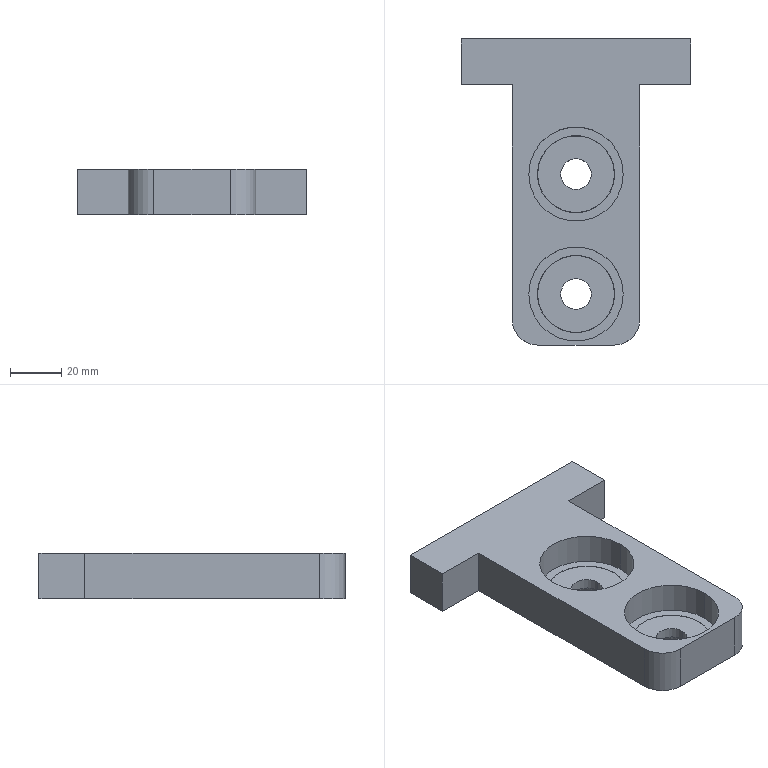Part | SolidWorks | features ICE 4, Fillet 3, Extrusion 1, LPattern 1 | 3 solids | 42 faces | box 90 x 120 x 18 mm | volume 92684 mm3 | cylinder 18 | plane 16 | torus 8 | commonest cylinder face diameters 12 x4 30.1 x4 30.3 x4 37 x4 20 x2
STEP:
#1=CARTESIAN_POINT('',(8.,-40.,0.));
#2=VERTEX_POINT('',#1);
#3=CARTESIAN_POINT('',(-8.,-40.,0.));
#4=VERTEX_POINT('',#3);
#5=CARTESIAN_POINT('',(0.,-40.,0.));
#6=DIRECTION('',(0.,0.,1.));
#7=DIRECTION('',(-1.,0.,0.));
#8=AXIS2_PLACEMENT_3D('',#5,#6,#7);
#9=CIRCLE('',#8,8.);
#10=EDGE_CURVE('',#2,#4,#9,.T.);
#11=ORIENTED_EDGE('',*,*,#10,.F.);
#12=CARTESIAN_POINT('',(6.,-40.,2.));
#13=VERTEX_POINT('',#12);
#14=CARTESIAN_POINT('',(8.,-40.,2.));
#15=DIRECTION('',(0.,1.,0.));
#16=DIRECTION('',(-1.,0.,0.));
#17=AXIS2_PLACEMENT_3D('',#14,#15,#16);
#18=CIRCLE('',#17,2.);
#19=EDGE_CURVE('',#2,#13,#18,.T.);
#20=ORIENTED_EDGE('',*,*,#19,.T.);
#21=CARTESIAN_POINT('',(-6.,-40.,2.));
#22=VERTEX_POINT('',#21);
#23=CARTESIAN_POINT('',(0.,-40.,2.));
#24=DIRECTION('',(0.,0.,-1.));
#25=DIRECTION('',(-1.,0.,0.));
#26=AXIS2_PLACEMENT_3D('',#23,#24,#25);
#27=CIRCLE('',#26,6.);
#28=EDGE_CURVE('',#22,#13,#27,.T.);
#29=ORIENTED_EDGE('',*,*,#28,.F.);
#30=CARTESIAN_POINT('',(-8.,-40.,2.));
#31=DIRECTION('',(0.,-1.,0.));
#32=DIRECTION('',(0.,0.,-1.));
#33=AXIS2_PLACEMENT_3D('',#30,#31,#32);
#34=CIRCLE('',#33,2.);
#35=EDGE_CURVE('',#4,#22,#34,.T.);
#36=ORIENTED_EDGE('',*,*,#35,.F.);
#37=EDGE_LOOP('',(#11,#20,#29,#36));
#38=FACE_OUTER_BOUND('',#37,.T.);
#39=CARTESIAN_POINT('',(0.,-40.,2.));
#40=DIRECTION('',(0.,0.,-1.));
#41=DIRECTION('',(-1.,0.,0.));
#42=AXIS2_PLACEMENT_3D('',#39,#40,#41);
#43=TOROIDAL_SURFACE('',#42,8.,2.);
#44=ADVANCED_FACE('',(#38),#43,.T.);
#45=CARTESIAN_POINT('',(15.05,-40.,2.));
#46=VERTEX_POINT('',#45);
#47=CARTESIAN_POINT('',(-15.05,-40.,2.));
#48=VERTEX_POINT('',#47);
#49=CARTESIAN_POINT('',(0.,-40.,2.));
#50=DIRECTION('',(0.,0.,1.));
#51=DIRECTION('',(-1.,0.,0.));
#52=AXIS2_PLACEMENT_3D('',#49,#50,#51);
#53=CIRCLE('',#52,15.05);
#54=EDGE_CURVE('',#46,#48,#53,.T.);
#55=ORIENTED_EDGE('',*,*,#54,.F.);
#56=CARTESIAN_POINT('',(13.05,-40.,0.));
#57=VERTEX_POINT('',#56);
#58=CARTESIAN_POINT('',(13.05,-40.,2.));
#59=DIRECTION('',(0.,1.,0.));
#60=DIRECTION('',(-1.,0.,0.));
#61=AXIS2_PLACEMENT_3D('',#58,#59,#60);
#62=CIRCLE('',#61,2.);
#63=EDGE_CURVE('',#46,#57,#62,.T.);
#64=ORIENTED_EDGE('',*,*,#63,.T.);
#65=CARTESIAN_POINT('',(-13.05,-40.,0.));
#66=VERTEX_POINT('',#65);
#67=CARTESIAN_POINT('',(0.,-40.,0.));
#68=DIRECTION('',(0.,0.,-1.));
#69=DIRECTION('',(-1.,0.,0.));
#70=AXIS2_PLACEMENT_3D('',#67,#68,#69);
#71=CIRCLE('',#70,13.05);
#72=EDGE_CURVE('',#66,#57,#71,.T.);
#73=ORIENTED_EDGE('',*,*,#72,.F.);
#74=CARTESIAN_POINT('',(-13.05,-40.,2.));
#75=DIRECTION('',(0.,-1.,0.));
#76=DIRECTION('',(0.,0.,-1.));
#77=AXIS2_PLACEMENT_3D('',#74,#75,#76);
#78=CIRCLE('',#77,2.);
#79=EDGE_CURVE('',#48,#66,#78,.T.);
#80=ORIENTED_EDGE('',*,*,#79,.F.);
#81=EDGE_LOOP('',(#55,#64,#73,#80));
#82=FACE_OUTER_BOUND('',#81,.T.);
#83=CARTESIAN_POINT('',(0.,-40.,2.));
#84=DIRECTION('',(0.,0.,-1.));
#85=DIRECTION('',(-1.,0.,0.));
#86=AXIS2_PLACEMENT_3D('',#83,#84,#85);
#87=TOROIDAL_SURFACE('',#86,13.05,2.);
#88=ADVANCED_FACE('',(#82),#87,.T.);
#89=CARTESIAN_POINT('',(15.05,-40.,6.));
#90=VERTEX_POINT('',#89);
#91=CARTESIAN_POINT('',(-15.05,-40.,6.));
#92=VERTEX_POINT('',#91);
#93=CARTESIAN_POINT('',(0.,-40.,6.));
#94=DIRECTION('',(0.,0.,1.));
#95=DIRECTION('',(-1.,0.,0.));
#96=AXIS2_PLACEMENT_3D('',#93,#94,#95);
#97=CIRCLE('',#96,15.05);
#98=EDGE_CURVE('',#90,#92,#97,.T.);
#99=ORIENTED_EDGE('',*,*,#98,.F.);
#100=CARTESIAN_POINT('',(15.05,-40.,18.));
#101=DIRECTION('',(0.,0.,-1.));
#102=VECTOR('',#101,1000.);
#103=LINE('',#100,#102);
#104=EDGE_CURVE('',#90,#46,#103,.T.);
#105=ORIENTED_EDGE('',*,*,#104,.T.);
#106=ORIENTED_EDGE('',*,*,#54,.T.);
#107=CARTESIAN_POINT('',(-15.05,-40.,18.));
#108=DIRECTION('',(0.,0.,-1.));
#109=VECTOR('',#108,1000.);
#110=LINE('',#107,#109);
#111=EDGE_CURVE('',#92,#48,#110,.T.);
#112=ORIENTED_EDGE('',*,*,#111,.F.);
#113=EDGE_LOOP('',(#99,#105,#106,#112));
#114=FACE_OUTER_BOUND('',#113,.T.);
#115=CARTESIAN_POINT('',(0.,-40.,18.));
#116=DIRECTION('',(0.,0.,-1.));
#117=DIRECTION('',(-1.,0.,0.));
#118=AXIS2_PLACEMENT_3D('',#115,#116,#117);
#119=CYLINDRICAL_SURFACE('',#118,15.05);
#120=ADVANCED_FACE('',(#114),#119,.T.);
#121=CARTESIAN_POINT('',(-6.,-40.,6.));
#122=VERTEX_POINT('',#121);
#123=CARTESIAN_POINT('',(6.,-40.,6.));
#124=VERTEX_POINT('',#123);
#125=CARTESIAN_POINT('',(0.,-40.,6.));
#126=DIRECTION('',(0.,0.,1.));
#127=DIRECTION('',(-1.,0.,0.));
#128=AXIS2_PLACEMENT_3D('',#125,#126,#127);
#129=CIRCLE('',#128,6.);
#130=EDGE_CURVE('',#122,#124,#129,.T.);
#131=ORIENTED_EDGE('',*,*,#130,.T.);
#132=CARTESIAN_POINT('',(6.,-40.,18.));
#133=DIRECTION('',(0.,0.,-1.));
#134=VECTOR('',#133,1000.);
#135=LINE('',#132,#134);
#136=EDGE_CURVE('',#124,#13,#135,.T.);
#137=ORIENTED_EDGE('',*,*,#136,.T.);
#138=CARTESIAN_POINT('',(0.,-40.,2.));
#139=DIRECTION('',(0.,0.,-1.));
#140=DIRECTION('',(-1.,0.,0.));
#141=AXIS2_PLACEMENT_3D('',#138,#139,#140);
#142=CIRCLE('',#141,6.);
#143=EDGE_CURVE('',#13,#22,#142,.T.);
#144=ORIENTED_EDGE('',*,*,#143,.T.);
#145=CARTESIAN_POINT('',(-6.,-40.,18.));
#146=DIRECTION('',(0.,0.,-1.));
#147=VECTOR('',#146,1000.);
#148=LINE('',#145,#147);
#149=EDGE_CURVE('',#122,#22,#148,.T.);
#150=ORIENTED_EDGE('',*,*,#149,.F.);
#151=EDGE_LOOP('',(#131,#137,#144,#150));
#152=FACE_OUTER_BOUND('',#151,.T.);
#153=CARTESIAN_POINT('',(0.,-40.,18.));
#154=DIRECTION('',(0.,0.,-1.));
#155=DIRECTION('',(-1.,0.,0.));
#156=AXIS2_PLACEMENT_3D('',#153,#154,#155);
#157=CYLINDRICAL_SURFACE('',#156,6.);
#158=ADVANCED_FACE('',(#152),#157,.F.);
#159=ORIENTED_EDGE('',*,*,#136,.F.);
#160=CARTESIAN_POINT('',(0.,-40.,6.));
#161=DIRECTION('',(0.,0.,1.));
#162=DIRECTION('',(-1.,0.,0.));
#163=AXIS2_PLACEMENT_3D('',#160,#161,#162);
#164=CIRCLE('',#163,6.);
#165=EDGE_CURVE('',#124,#122,#164,.T.);
#166=ORIENTED_EDGE('',*,*,#165,.T.);
#167=ORIENTED_EDGE('',*,*,#149,.T.);
#168=ORIENTED_EDGE('',*,*,#28,.T.);
#169=EDGE_LOOP('',(#159,#166,#167,#168));
#170=FACE_OUTER_BOUND('',#169,.T.);
#171=CARTESIAN_POINT('',(0.,-40.,18.));
#172=DIRECTION('',(0.,0.,-1.));
#173=DIRECTION('',(-1.,0.,0.));
#174=AXIS2_PLACEMENT_3D('',#171,#172,#173);
#175=CYLINDRICAL_SURFACE('',#174,6.);
#176=ADVANCED_FACE('',(#170),#175,.F.);
#177=ORIENTED_EDGE('',*,*,#72,.T.);
#178=CARTESIAN_POINT('',(0.,-40.,0.));
#179=DIRECTION('',(0.,0.,-1.));
#180=DIRECTION('',(-1.,0.,0.));
#181=AXIS2_PLACEMENT_3D('',#178,#179,#180);
#182=CIRCLE('',#181,13.05);
#183=EDGE_CURVE('',#57,#66,#182,.T.);
#184=ORIENTED_EDGE('',*,*,#183,.T.);
#185=EDGE_LOOP('',(#177,#184));
#186=FACE_OUTER_BOUND('',#185,.T.);
#187=CARTESIAN_POINT('',(0.,-40.,0.));
#188=DIRECTION('',(0.,0.,1.));
#189=DIRECTION('',(-1.,0.,0.));
#190=AXIS2_PLACEMENT_3D('',#187,#188,#189);
#191=CIRCLE('',#190,8.);
#192=EDGE_CURVE('',#4,#2,#191,.T.);
#193=ORIENTED_EDGE('',*,*,#192,.T.);
#194=ORIENTED_EDGE('',*,*,#10,.T.);
#195=EDGE_LOOP('',(#193,#194));
#196=FACE_BOUND('',#195,.T.);
#197=CARTESIAN_POINT('',(0.,0.,0.));
#198=DIRECTION('',(0.,0.,-1.));
#199=DIRECTION('',(-1.,0.,0.));
#200=AXIS2_PLACEMENT_3D('',#197,#198,#199);
#201=PLANE('',#200);
#202=ADVANCED_FACE('',(#186,#196),#201,.T.);
#203=ORIENTED_EDGE('',*,*,#104,.F.);
#204=CARTESIAN_POINT('',(0.,-40.,6.));
#205=DIRECTION('',(0.,0.,1.));
#206=DIRECTION('',(-1.,0.,0.));
#207=AXIS2_PLACEMENT_3D('',#204,#205,#206);
#208=CIRCLE('',#207,15.05);
#209=EDGE_CURVE('',#92,#90,#208,.T.);
#210=ORIENTED_EDGE('',*,*,#209,.F.);
#211=ORIENTED_EDGE('',*,*,#111,.T.);
#212=CARTESIAN_POINT('',(0.,-40.,2.));
#213=DIRECTION('',(0.,0.,1.));
#214=DIRECTION('',(-1.,0.,0.));
#215=AXIS2_PLACEMENT_3D('',#212,#213,#214);
#216=CIRCLE('',#215,15.05);
#217=EDGE_CURVE('',#48,#46,#216,.T.);
#218=ORIENTED_EDGE('',*,*,#217,.T.);
#219=EDGE_LOOP('',(#203,#210,#211,#218));
#220=FACE_OUTER_BOUND('',#219,.T.);
#221=CARTESIAN_POINT('',(0.,-40.,18.));
#222=DIRECTION('',(0.,0.,-1.));
#223=DIRECTION('',(-1.,0.,0.));
#224=AXIS2_PLACEMENT_3D('',#221,#222,#223);
#225=CYLINDRICAL_SURFACE('',#224,15.05);
#226=ADVANCED_FACE('',(#220),#225,.T.);
#227=ORIENTED_EDGE('',*,*,#63,.F.);
#228=ORIENTED_EDGE('',*,*,#217,.F.);
#229=ORIENTED_EDGE('',*,*,#79,.T.);
#230=ORIENTED_EDGE('',*,*,#183,.F.);
#231=EDGE_LOOP('',(#227,#228,#229,#230));
#232=FACE_OUTER_BOUND('',#231,.T.);
#233=CARTESIAN_POINT('',(0.,-40.,2.));
#234=DIRECTION('',(0.,0.,-1.));
#235=DIRECTION('',(-1.,0.,0.));
#236=AXIS2_PLACEMENT_3D('',#233,#234,#235);
#237=TOROIDAL_SURFACE('',#236,13.05,2.);
#238=ADVANCED_FACE('',(#232),#237,.T.);
#239=ORIENTED_EDGE('',*,*,#19,.F.);
#240=ORIENTED_EDGE('',*,*,#192,.F.);
#241=ORIENTED_EDGE('',*,*,#35,.T.);
#242=ORIENTED_EDGE('',*,*,#143,.F.);
#243=EDGE_LOOP('',(#239,#240,#241,#242));
#244=FACE_OUTER_BOUND('',#243,.T.);
#245=CARTESIAN_POINT('',(0.,-40.,2.));
#246=DIRECTION('',(0.,0.,-1.));
#247=DIRECTION('',(-1.,0.,0.));
#248=AXIS2_PLACEMENT_3D('',#245,#246,#247);
#249=TOROIDAL_SURFACE('',#248,8.,2.);
#250=ADVANCED_FACE('',(#244),#249,.T.);
#251=ORIENTED_EDGE('',*,*,#209,.T.);
#252=ORIENTED_EDGE('',*,*,#98,.T.);
#253=EDGE_LOOP('',(#251,#252));
#254=FACE_OUTER_BOUND('',#253,.T.);
#255=ORIENTED_EDGE('',*,*,#130,.F.);
#256=ORIENTED_EDGE('',*,*,#165,.F.);
#257=EDGE_LOOP('',(#255,#256));
#258=FACE_BOUND('',#257,.T.);
#259=CARTESIAN_POINT('',(0.,-40.,6.));
#260=DIRECTION('',(0.,0.,-1.));
#261=DIRECTION('',(-1.,0.,0.));
#262=AXIS2_PLACEMENT_3D('',#259,#260,#261);
#263=PLANE('',#262);
#264=ADVANCED_FACE('',(#254,#258),#263,.F.);
#265=CLOSED_SHELL('',(#44,#88,#120,#158,#176,#202,#226,#238,#250,#264));
#266=MANIFOLD_SOLID_BREP('',#265);
#267=CARTESIAN_POINT('',(18.5,-40.,6.));
#268=VERTEX_POINT('',#267);
#269=CARTESIAN_POINT('',(-18.5,-40.,6.));
#270=VERTEX_POINT('',#269);
#271=CARTESIAN_POINT('',(0.,-40.,6.));
#272=DIRECTION('',(0.,0.,-1.));
#273=DIRECTION('',(-1.,0.,0.));
#274=AXIS2_PLACEMENT_3D('',#271,#272,#273);
#275=CIRCLE('',#274,18.5);
#276=EDGE_CURVE('',#268,#270,#275,.T.);
#277=ORIENTED_EDGE('',*,*,#276,.T.);
#278=CARTESIAN_POINT('',(-18.5,-40.,18.));
#279=VERTEX_POINT('',#278);
#280=CARTESIAN_POINT('',(-18.5,-40.,6.));
#281=DIRECTION('',(0.,0.,1.));
#282=VECTOR('',#281,1000.);
#283=LINE('',#280,#282);
#284=EDGE_CURVE('',#270,#279,#283,.T.);
#285=ORIENTED_EDGE('',*,*,#284,.T.);
#286=CARTESIAN_POINT('',(18.5,-40.,18.));
#287=VERTEX_POINT('',#286);
#288=CARTESIAN_POINT('',(0.,-40.,18.));
#289=DIRECTION('',(0.,0.,-1.));
#290=DIRECTION('',(-1.,0.,0.));
#291=AXIS2_PLACEMENT_3D('',#288,#289,#290);
#292=CIRCLE('',#291,18.5);
#293=EDGE_CURVE('',#287,#279,#292,.T.);
#294=ORIENTED_EDGE('',*,*,#293,.F.);
#295=CARTESIAN_POINT('',(18.5,-40.,6.));
#296=DIRECTION('',(0.,0.,1.));
#297=VECTOR('',#296,1000.);
#298=LINE('',#295,#297);
#299=EDGE_CURVE('',#268,#287,#298,.T.);
#300=ORIENTED_EDGE('',*,*,#299,.F.);
#301=EDGE_LOOP('',(#277,#285,#294,#300));
#302=FACE_OUTER_BOUND('',#301,.T.);
#303=CARTESIAN_POINT('',(0.,-40.,6.));
#304=DIRECTION('',(0.,0.,1.));
#305=DIRECTION('',(1.,0.,0.));
#306=AXIS2_PLACEMENT_3D('',#303,#304,#305);
#307=CYLINDRICAL_SURFACE('',#306,18.5);
#308=ADVANCED_FACE('',(#302),#307,.F.);
#309=CARTESIAN_POINT('',(18.5,7.,6.));
#310=VERTEX_POINT('',#309);
#311=CARTESIAN_POINT('',(-18.5,7.,6.));
#312=VERTEX_POINT('',#311);
#313=CARTESIAN_POINT('',(0.,7.,6.));
#314=DIRECTION('',(0.,0.,-1.));
#315=DIRECTION('',(-1.,0.,0.));
#316=AXIS2_PLACEMENT_3D('',#313,#314,#315);
#317=CIRCLE('',#316,18.5);
#318=EDGE_CURVE('',#310,#312,#317,.T.);
#319=ORIENTED_EDGE('',*,*,#318,.T.);
#320=CARTESIAN_POINT('',(-18.5,7.,18.));
#321=VERTEX_POINT('',#320);
#322=CARTESIAN_POINT('',(-18.5,7.,6.));
#323=DIRECTION('',(0.,0.,1.));
#324=VECTOR('',#323,1000.);
#325=LINE('',#322,#324);
#326=EDGE_CURVE('',#312,#321,#325,.T.);
#327=ORIENTED_EDGE('',*,*,#326,.T.);
#328=CARTESIAN_POINT('',(18.5,7.,18.));
#329=VERTEX_POINT('',#328);
#330=CARTESIAN_POINT('',(0.,7.,18.));
#331=DIRECTION('',(0.,0.,-1.));
#332=DIRECTION('',(-1.,0.,0.));
#333=AXIS2_PLACEMENT_3D('',#330,#331,#332);
#334=CIRCLE('',#333,18.5);
#335=EDGE_CURVE('',#329,#321,#334,.T.);
#336=ORIENTED_EDGE('',*,*,#335,.F.);
#337=CARTESIAN_POINT('',(18.5,7.,6.));
#338=DIRECTION('',(0.,0.,1.));
#339=VECTOR('',#338,1000.);
#340=LINE('',#337,#339);
#341=EDGE_CURVE('',#310,#329,#340,.T.);
#342=ORIENTED_EDGE('',*,*,#341,.F.);
#343=EDGE_LOOP('',(#319,#327,#336,#342));
#344=FACE_OUTER_BOUND('',#343,.T.);
#345=CARTESIAN_POINT('',(0.,7.,6.));
#346=DIRECTION('',(0.,0.,1.));
#347=DIRECTION('',(1.,0.,0.));
#348=AXIS2_PLACEMENT_3D('',#345,#346,#347);
#349=CYLINDRICAL_SURFACE('',#348,18.5);
#350=ADVANCED_FACE('',(#344),#349,.F.);
#351=CARTESIAN_POINT('',(-15.15,7.,6.));
#352=VERTEX_POINT('',#351);
#353=CARTESIAN_POINT('',(15.15,7.,6.));
#354=VERTEX_POINT('',#353);
#355=CARTESIAN_POINT('',(0.,7.,6.));
#356=DIRECTION('',(0.,0.,1.));
#357=DIRECTION('',(-1.,0.,0.));
#358=AXIS2_PLACEMENT_3D('',#355,#356,#357);
#359=CIRCLE('',#358,15.15);
#360=EDGE_CURVE('',#352,#354,#359,.T.);
#361=ORIENTED_EDGE('',*,*,#360,.T.);
#362=CARTESIAN_POINT('',(15.15,7.,0.));
#363=VERTEX_POINT('',#362);
#364=CARTESIAN_POINT('',(15.15,7.,18.));
#365=DIRECTION('',(0.,0.,-1.));
#366=VECTOR('',#365,1000.);
#367=LINE('',#364,#366);
#368=EDGE_CURVE('',#354,#363,#367,.T.);
#369=ORIENTED_EDGE('',*,*,#368,.T.);
#370=CARTESIAN_POINT('',(-15.15,7.,0.));
#371=VERTEX_POINT('',#370);
#372=CARTESIAN_POINT('',(0.,7.,0.));
#373=DIRECTION('',(0.,0.,-1.));
#374=DIRECTION('',(-1.,0.,0.));
#375=AXIS2_PLACEMENT_3D('',#372,#373,#374);
#376=CIRCLE('',#375,15.15);
#377=EDGE_CURVE('',#363,#371,#376,.T.);
#378=ORIENTED_EDGE('',*,*,#377,.T.);
#379=CARTESIAN_POINT('',(-15.15,7.,18.));
#380=DIRECTION('',(0.,0.,-1.));
#381=VECTOR('',#380,1000.);
#382=LINE('',#379,#381);
#383=EDGE_CURVE('',#352,#371,#382,.T.);
#384=ORIENTED_EDGE('',*,*,#383,.F.);
#385=EDGE_LOOP('',(#361,#369,#378,#384));
#386=FACE_OUTER_BOUND('',#385,.T.);
#387=CARTESIAN_POINT('',(0.,7.,18.));
#388=DIRECTION('',(0.,0.,-1.));
#389=DIRECTION('',(-1.,0.,0.));
#390=AXIS2_PLACEMENT_3D('',#387,#388,#389);
#391=CYLINDRICAL_SURFACE('',#390,15.15);
#392=ADVANCED_FACE('',(#386),#391,.F.);
#393=CARTESIAN_POINT('',(-15.15,-40.,6.));
#394=VERTEX_POINT('',#393);
#395=CARTESIAN_POINT('',(15.15,-40.,6.));
#396=VERTEX_POINT('',#395);
#397=CARTESIAN_POINT('',(0.,-40.,6.));
#398=DIRECTION('',(0.,0.,1.));
#399=DIRECTION('',(-1.,0.,0.));
#400=AXIS2_PLACEMENT_3D('',#397,#398,#399);
#401=CIRCLE('',#400,15.15);
#402=EDGE_CURVE('',#394,#396,#401,.T.);
#403=ORIENTED_EDGE('',*,*,#402,.T.);
#404=CARTESIAN_POINT('',(15.15,-40.,0.));
#405=VERTEX_POINT('',#404);
#406=CARTESIAN_POINT('',(15.15,-40.,18.));
#407=DIRECTION('',(0.,0.,-1.));
#408=VECTOR('',#407,1000.);
#409=LINE('',#406,#408);
#410=EDGE_CURVE('',#396,#405,#409,.T.);
#411=ORIENTED_EDGE('',*,*,#410,.T.);
#412=CARTESIAN_POINT('',(-15.15,-40.,0.));
#413=VERTEX_POINT('',#412);
#414=CARTESIAN_POINT('',(0.,-40.,0.));
#415=DIRECTION('',(0.,0.,-1.));
#416=DIRECTION('',(-1.,0.,0.));
#417=AXIS2_PLACEMENT_3D('',#414,#415,#416);
#418=CIRCLE('',#417,15.15);
#419=EDGE_CURVE('',#405,#413,#418,.T.);
#420=ORIENTED_EDGE('',*,*,#419,.T.);
#421=CARTESIAN_POINT('',(-15.15,-40.,18.));
#422=DIRECTION('',(0.,0.,-1.));
#423=VECTOR('',#422,1000.);
#424=LINE('',#421,#423);
#425=EDGE_CURVE('',#394,#413,#424,.T.);
#426=ORIENTED_EDGE('',*,*,#425,.F.);
#427=EDGE_LOOP('',(#403,#411,#420,#426));
#428=FACE_OUTER_BOUND('',#427,.T.);
#429=CARTESIAN_POINT('',(0.,-40.,18.));
#430=DIRECTION('',(0.,0.,-1.));
#431=DIRECTION('',(-1.,0.,0.));
#432=AXIS2_PLACEMENT_3D('',#429,#430,#431);
#433=CYLINDRICAL_SURFACE('',#432,15.15);
#434=ADVANCED_FACE('',(#428),#433,.F.);
#435=CARTESIAN_POINT('',(-25.,42.,0.));
#436=VERTEX_POINT('',#435);
#437=CARTESIAN_POINT('',(-25.,-50.,0.));
#438=VERTEX_POINT('',#437);
#439=CARTESIAN_POINT('',(-25.,60.,0.));
#440=DIRECTION('',(0.,-1.,0.));
#441=VECTOR('',#440,1000.);
#442=LINE('',#439,#441);
#443=EDGE_CURVE('',#436,#438,#442,.T.);
#444=ORIENTED_EDGE('',*,*,#443,.T.);
#445=CARTESIAN_POINT('',(-25.,-50.,18.));
#446=VERTEX_POINT('',#445);
#447=CARTESIAN_POINT('',(-25.,-50.,18.));
#448=DIRECTION('',(0.,0.,1.));
#449=VECTOR('',#448,1000.);
#450=LINE('',#447,#449);
#451=EDGE_CURVE('',#438,#446,#450,.T.);
#452=ORIENTED_EDGE('',*,*,#451,.T.);
#453=CARTESIAN_POINT('',(-25.,42.,18.));
#454=VERTEX_POINT('',#453);
#455=CARTESIAN_POINT('',(-25.,60.,18.));
#456=DIRECTION('',(0.,-1.,0.));
#457=VECTOR('',#456,1000.);
#458=LINE('',#455,#457);
#459=EDGE_CURVE('',#454,#446,#458,.T.);
#460=ORIENTED_EDGE('',*,*,#459,.F.);
#461=CARTESIAN_POINT('',(-25.,42.,18.));
#462=DIRECTION('',(0.,0.,1.));
#463=VECTOR('',#462,1000.);
#464=LINE('',#461,#463);
#465=EDGE_CURVE('',#436,#454,#464,.T.);
#466=ORIENTED_EDGE('',*,*,#465,.F.);
#467=EDGE_LOOP('',(#444,#452,#460,#466));
#468=FACE_OUTER_BOUND('',#467,.T.);
#469=CARTESIAN_POINT('',(-25.,60.,18.));
#470=DIRECTION('',(1.,0.,0.));
#471=DIRECTION('',(0.,1.,0.));
#472=AXIS2_PLACEMENT_3D('',#469,#470,#471);
#473=PLANE('',#472);
#474=ADVANCED_FACE('',(#468),#473,.F.);
#475=CARTESIAN_POINT('',(25.,-50.,18.));
#476=VERTEX_POINT('',#475);
#477=CARTESIAN_POINT('',(25.,42.,18.));
#478=VERTEX_POINT('',#477);
#479=CARTESIAN_POINT('',(25.,60.,18.));
#480=DIRECTION('',(0.,1.,0.));
#481=VECTOR('',#480,1000.);
#482=LINE('',#479,#481);
#483=EDGE_CURVE('',#476,#478,#482,.T.);
#484=ORIENTED_EDGE('',*,*,#483,.F.);
#485=CARTESIAN_POINT('',(25.,-50.,0.));
#486=VERTEX_POINT('',#485);
#487=CARTESIAN_POINT('',(25.,-50.,18.));
#488=DIRECTION('',(0.,0.,-1.));
#489=VECTOR('',#488,1000.);
#490=LINE('',#487,#489);
#491=EDGE_CURVE('',#476,#486,#490,.T.);
#492=ORIENTED_EDGE('',*,*,#491,.T.);
#493=CARTESIAN_POINT('',(25.,42.,0.));
#494=VERTEX_POINT('',#493);
#495=CARTESIAN_POINT('',(25.,60.,0.));
#496=DIRECTION('',(0.,1.,0.));
#497=VECTOR('',#496,1000.);
#498=LINE('',#495,#497);
#499=EDGE_CURVE('',#486,#494,#498,.T.);
#500=ORIENTED_EDGE('',*,*,#499,.T.);
#501=CARTESIAN_POINT('',(25.,42.,18.));
#502=DIRECTION('',(0.,0.,-1.));
#503=VECTOR('',#502,1000.);
#504=LINE('',#501,#503);
#505=EDGE_CURVE('',#478,#494,#504,.T.);
#506=ORIENTED_EDGE('',*,*,#505,.F.);
#507=EDGE_LOOP('',(#484,#492,#500,#506));
#508=FACE_OUTER_BOUND('',#507,.T.);
#509=CARTESIAN_POINT('',(25.,60.,18.));
#510=DIRECTION('',(-1.,0.,0.));
#511=DIRECTION('',(0.,-1.,0.));
#512=AXIS2_PLACEMENT_3D('',#509,#510,#511);
#513=PLANE('',#512);
#514=ADVANCED_FACE('',(#508),#513,.F.);
#515=CARTESIAN_POINT('',(-15.,-60.,0.));
#516=VERTEX_POINT('',#515);
#517=CARTESIAN_POINT('',(15.,-60.,0.));
#518=VERTEX_POINT('',#517);
#519=CARTESIAN_POINT('',(25.,-60.,0.));
#520=DIRECTION('',(1.,0.,0.));
#521=VECTOR('',#520,1000.);
#522=LINE('',#519,#521);
#523=EDGE_CURVE('',#516,#518,#522,.T.);
#524=ORIENTED_EDGE('',*,*,#523,.T.);
#525=CARTESIAN_POINT('',(15.,-60.,18.));
#526=VERTEX_POINT('',#525);
#527=CARTESIAN_POINT('',(15.,-60.,18.));
#528=DIRECTION('',(0.,0.,1.));
#529=VECTOR('',#528,1000.);
#530=LINE('',#527,#529);
#531=EDGE_CURVE('',#518,#526,#530,.T.);
#532=ORIENTED_EDGE('',*,*,#531,.T.);
#533=CARTESIAN_POINT('',(-15.,-60.,18.));
#534=VERTEX_POINT('',#533);
#535=CARTESIAN_POINT('',(25.,-60.,18.));
#536=DIRECTION('',(1.,0.,0.));
#537=VECTOR('',#536,1000.);
#538=LINE('',#535,#537);
#539=EDGE_CURVE('',#534,#526,#538,.T.);
#540=ORIENTED_EDGE('',*,*,#539,.F.);
#541=CARTESIAN_POINT('',(-15.,-60.,18.));
#542=DIRECTION('',(0.,0.,-1.));
#543=VECTOR('',#542,1000.);
#544=LINE('',#541,#543);
#545=EDGE_CURVE('',#534,#516,#544,.T.);
#546=ORIENTED_EDGE('',*,*,#545,.T.);
#547=EDGE_LOOP('',(#524,#532,#540,#546));
#548=FACE_OUTER_BOUND('',#547,.T.);
#549=CARTESIAN_POINT('',(25.,-60.,18.));
#550=DIRECTION('',(0.,1.,0.));
#551=DIRECTION('',(0.,0.,1.));
#552=AXIS2_PLACEMENT_3D('',#549,#550,#551);
#553=PLANE('',#552);
#554=ADVANCED_FACE('',(#548),#553,.F.);
#555=CARTESIAN_POINT('',(45.,60.,0.));
#556=VERTEX_POINT('',#555);
#557=CARTESIAN_POINT('',(-45.,60.,0.));
#558=VERTEX_POINT('',#557);
#559=CARTESIAN_POINT('',(25.,60.,0.));
#560=DIRECTION('',(-1.,0.,0.));
#561=VECTOR('',#560,1000.);
#562=LINE('',#559,#561);
#563=EDGE_CURVE('',#556,#558,#562,.T.);
#564=ORIENTED_EDGE('',*,*,#563,.T.);
#565=CARTESIAN_POINT('',(-45.,60.,18.));
#566=VERTEX_POINT('',#565);
#567=CARTESIAN_POINT('',(-45.,60.,18.));
#568=DIRECTION('',(0.,0.,1.));
#569=VECTOR('',#568,1000.);
#570=LINE('',#567,#569);
#571=EDGE_CURVE('',#558,#566,#570,.T.);
#572=ORIENTED_EDGE('',*,*,#571,.T.);
#573=CARTESIAN_POINT('',(45.,60.,18.));
#574=VERTEX_POINT('',#573);
#575=CARTESIAN_POINT('',(25.,60.,18.));
#576=DIRECTION('',(-1.,0.,0.));
#577=VECTOR('',#576,1000.);
#578=LINE('',#575,#577);
#579=EDGE_CURVE('',#574,#566,#578,.T.);
#580=ORIENTED_EDGE('',*,*,#579,.F.);
#581=CARTESIAN_POINT('',(45.,60.,18.));
#582=DIRECTION('',(0.,0.,-1.));
#583=VECTOR('',#582,1000.);
#584=LINE('',#581,#583);
#585=EDGE_CURVE('',#574,#556,#584,.T.);
#586=ORIENTED_EDGE('',*,*,#585,.T.);
#587=EDGE_LOOP('',(#564,#572,#580,#586));
#588=FACE_OUTER_BOUND('',#587,.T.);
#589=CARTESIAN_POINT('',(25.,60.,18.));
#590=DIRECTION('',(0.,-1.,0.));
#591=DIRECTION('',(0.,0.,-1.));
#592=AXIS2_PLACEMENT_3D('',#589,#590,#591);
#593=PLANE('',#592);
#594=ADVANCED_FACE('',(#588),#593,.F.);
#595=ORIENTED_EDGE('',*,*,#293,.T.);
#596=CARTESIAN_POINT('',(0.,-40.,18.));
#597=DIRECTION('',(0.,0.,-1.));
#598=DIRECTION('',(-1.,0.,0.));
#599=AXIS2_PLACEMENT_3D('',#596,#597,#598);
#600=CIRCLE('',#599,18.5);
#601=EDGE_CURVE('',#279,#287,#600,.T.);
#602=ORIENTED_EDGE('',*,*,#601,.T.);
#603=EDGE_LOOP('',(#595,#602));
#604=FACE_BOUND('',#603,.T.);
#605=ORIENTED_EDGE('',*,*,#335,.T.);
#606=CARTESIAN_POINT('',(0.,7.,18.));
#607=DIRECTION('',(0.,0.,-1.));
#608=DIRECTION('',(-1.,0.,0.));
#609=AXIS2_PLACEMENT_3D('',#606,#607,#608);
#610=CIRCLE('',#609,18.5);
#611=EDGE_CURVE('',#321,#329,#610,.T.);
#612=ORIENTED_EDGE('',*,*,#611,.T.);
#613=EDGE_LOOP('',(#605,#612));
#614=FACE_BOUND('',#613,.T.);
#615=ORIENTED_EDGE('',*,*,#539,.T.);
#616=CARTESIAN_POINT('',(15.,-50.,18.));
#617=DIRECTION('',(0.,0.,1.));
#618=DIRECTION('',(-1.,0.,0.));
#619=AXIS2_PLACEMENT_3D('',#616,#617,#618);
#620=CIRCLE('',#619,10.);
#621=EDGE_CURVE('',#526,#476,#620,.T.);
#622=ORIENTED_EDGE('',*,*,#621,.T.);
#623=ORIENTED_EDGE('',*,*,#483,.T.);
#624=CARTESIAN_POINT('',(45.,42.,18.));
#625=VERTEX_POINT('',#624);
#626=CARTESIAN_POINT('',(45.,42.,18.));
#627=DIRECTION('',(1.,0.,0.));
#628=VECTOR('',#627,1000.);
#629=LINE('',#626,#628);
#630=EDGE_CURVE('',#478,#625,#629,.T.);
#631=ORIENTED_EDGE('',*,*,#630,.T.);
#632=CARTESIAN_POINT('',(45.,42.,18.));
#633=DIRECTION('',(0.,1.,0.));
#634=VECTOR('',#633,1000.);
#635=LINE('',#632,#634);
#636=EDGE_CURVE('',#625,#574,#635,.T.);
#637=ORIENTED_EDGE('',*,*,#636,.T.);
#638=ORIENTED_EDGE('',*,*,#579,.T.);
#639=CARTESIAN_POINT('',(-45.,42.,18.));
#640=VERTEX_POINT('',#639);
#641=CARTESIAN_POINT('',(-45.,42.,18.));
#642=DIRECTION('',(0.,1.,0.));
#643=VECTOR('',#642,1000.);
#644=LINE('',#641,#643);
#645=EDGE_CURVE('',#640,#566,#644,.T.);
#646=ORIENTED_EDGE('',*,*,#645,.F.);
#647=CARTESIAN_POINT('',(45.,42.,18.));
#648=DIRECTION('',(1.,0.,0.));
#649=VECTOR('',#648,1000.);
#650=LINE('',#647,#649);
#651=EDGE_CURVE('',#640,#454,#650,.T.);
#652=ORIENTED_EDGE('',*,*,#651,.T.);
#653=ORIENTED_EDGE('',*,*,#459,.T.);
#654=CARTESIAN_POINT('',(-15.,-50.,18.));
#655=DIRECTION('',(0.,0.,1.));
#656=DIRECTION('',(-1.,0.,0.));
#657=AXIS2_PLACEMENT_3D('',#654,#655,#656);
#658=CIRCLE('',#657,10.);
#659=EDGE_CURVE('',#446,#534,#658,.T.);
#660=ORIENTED_EDGE('',*,*,#659,.T.);
#661=EDGE_LOOP('',(#615,#622,#623,#631,#637,#638,#646,#652,#653,#660));
#662=FACE_OUTER_BOUND('',#661,.T.);
#663=CARTESIAN_POINT('',(0.,0.,18.));
#664=DIRECTION('',(0.,0.,-1.));
#665=DIRECTION('',(-1.,0.,0.));
#666=AXIS2_PLACEMENT_3D('',#663,#664,#665);
#667=PLANE('',#666);
#668=ADVANCED_FACE('',(#604,#614,#662),#667,.F.);
#669=CARTESIAN_POINT('',(0.,7.,0.));
#670=DIRECTION('',(0.,0.,-1.));
#671=DIRECTION('',(-1.,0.,0.));
#672=AXIS2_PLACEMENT_3D('',#669,#670,#671);
#673=CIRCLE('',#672,15.15);
#674=EDGE_CURVE('',#371,#363,#673,.T.);
#675=ORIENTED_EDGE('',*,*,#674,.F.);
#676=ORIENTED_EDGE('',*,*,#377,.F.);
#677=EDGE_LOOP('',(#675,#676));
#678=FACE_BOUND('',#677,.T.);
#679=CARTESIAN_POINT('',(0.,-40.,0.));
#680=DIRECTION('',(0.,0.,-1.));
#681=DIRECTION('',(-1.,0.,0.));
#682=AXIS2_PLACEMENT_3D('',#679,#680,#681);
#683=CIRCLE('',#682,15.15);
#684=EDGE_CURVE('',#413,#405,#683,.T.);
#685=ORIENTED_EDGE('',*,*,#684,.F.);
#686=ORIENTED_EDGE('',*,*,#419,.F.);
#687=EDGE_LOOP('',(#685,#686));
#688=FACE_BOUND('',#687,.T.);
#689=ORIENTED_EDGE('',*,*,#499,.F.);
#690=CARTESIAN_POINT('',(15.,-50.,0.));
#691=DIRECTION('',(0.,0.,-1.));
#692=DIRECTION('',(-1.,0.,0.));
#693=AXIS2_PLACEMENT_3D('',#690,#691,#692);
#694=CIRCLE('',#693,10.);
#695=EDGE_CURVE('',#486,#518,#694,.T.);
#696=ORIENTED_EDGE('',*,*,#695,.T.);
#697=ORIENTED_EDGE('',*,*,#523,.F.);
#698=CARTESIAN_POINT('',(-15.,-50.,0.));
#699=DIRECTION('',(0.,0.,-1.));
#700=DIRECTION('',(-1.,0.,0.));
#701=AXIS2_PLACEMENT_3D('',#698,#699,#700);
#702=CIRCLE('',#701,10.);
#703=EDGE_CURVE('',#516,#438,#702,.T.);
#704=ORIENTED_EDGE('',*,*,#703,.T.);
#705=ORIENTED_EDGE('',*,*,#443,.F.);
#706=CARTESIAN_POINT('',(-45.,42.,0.));
#707=VERTEX_POINT('',#706);
#708=CARTESIAN_POINT('',(45.,42.,0.));
#709=DIRECTION('',(-1.,0.,0.));
#710=VECTOR('',#709,1000.);
#711=LINE('',#708,#710);
#712=EDGE_CURVE('',#436,#707,#711,.T.);
#713=ORIENTED_EDGE('',*,*,#712,.T.);
#714=CARTESIAN_POINT('',(-45.,42.,0.));
#715=DIRECTION('',(0.,1.,0.));
#716=VECTOR('',#715,1000.);
#717=LINE('',#714,#716);
#718=EDGE_CURVE('',#707,#558,#717,.T.);
#719=ORIENTED_EDGE('',*,*,#718,.T.);
#720=ORIENTED_EDGE('',*,*,#563,.F.);
#721=CARTESIAN_POINT('',(45.,42.,0.));
#722=VERTEX_POINT('',#721);
#723=CARTESIAN_POINT('',(45.,42.,0.));
#724=DIRECTION('',(0.,1.,0.));
#725=VECTOR('',#724,1000.);
#726=LINE('',#723,#725);
#727=EDGE_CURVE('',#722,#556,#726,.T.);
#728=ORIENTED_EDGE('',*,*,#727,.F.);
#729=CARTESIAN_POINT('',(45.,42.,0.));
#730=DIRECTION('',(-1.,0.,0.));
#731=VECTOR('',#730,1000.);
#732=LINE('',#729,#731);
#733=EDGE_CURVE('',#722,#494,#732,.T.);
#734=ORIENTED_EDGE('',*,*,#733,.T.);
#735=EDGE_LOOP('',(#689,#696,#697,#704,#705,#713,#719,#720,#728,#734));
#736=FACE_OUTER_BOUND('',#735,.T.);
#737=CARTESIAN_POINT('',(0.,0.,0.));
#738=DIRECTION('',(0.,0.,-1.));
#739=DIRECTION('',(-1.,0.,0.));
#740=AXIS2_PLACEMENT_3D('',#737,#738,#739);
#741=PLANE('',#740);
#742=ADVANCED_FACE('',(#678,#688,#736),#741,.T.);
#743=ORIENTED_EDGE('',*,*,#585,.F.);
#744=ORIENTED_EDGE('',*,*,#636,.F.);
#745=CARTESIAN_POINT('',(45.,42.,18.));
#746=DIRECTION('',(0.,0.,-1.));
#747=VECTOR('',#746,1000.);
#748=LINE('',#745,#747);
#749=EDGE_CURVE('',#625,#722,#748,.T.);
#750=ORIENTED_EDGE('',*,*,#749,.T.);
#751=ORIENTED_EDGE('',*,*,#727,.T.);
#752=EDGE_LOOP('',(#743,#744,#750,#751));
#753=FACE_OUTER_BOUND('',#752,.T.);
#754=CARTESIAN_POINT('',(45.,42.,18.));
#755=DIRECTION('',(1.,0.,0.));
#756=DIRECTION('',(0.,0.,-1.));
#757=AXIS2_PLACEMENT_3D('',#754,#755,#756);
#758=PLANE('',#757);
#759=ADVANCED_FACE('',(#753),#758,.T.);
#760=ORIENTED_EDGE('',*,*,#630,.F.);
#761=ORIENTED_EDGE('',*,*,#505,.T.);
#762=ORIENTED_EDGE('',*,*,#733,.F.);
#763=ORIENTED_EDGE('',*,*,#749,.F.);
#764=EDGE_LOOP('',(#760,#761,#762,#763));
#765=FACE_OUTER_BOUND('',#764,.T.);
#766=CARTESIAN_POINT('',(0.,42.,0.));
#767=DIRECTION('',(0.,1.,0.));
#768=DIRECTION('',(0.,0.,1.));
#769=AXIS2_PLACEMENT_3D('',#766,#767,#768);
#770=PLANE('',#769);
#771=ADVANCED_FACE('',(#765),#770,.F.);
#772=ORIENTED_EDGE('',*,*,#712,.F.);
#773=ORIENTED_EDGE('',*,*,#465,.T.);
#774=ORIENTED_EDGE('',*,*,#651,.F.);
#775=CARTESIAN_POINT('',(-45.,42.,18.));
#776=DIRECTION('',(0.,0.,1.));
#777=VECTOR('',#776,1000.);
#778=LINE('',#775,#777);
#779=EDGE_CURVE('',#707,#640,#778,.T.);
#780=ORIENTED_EDGE('',*,*,#779,.F.);
#781=EDGE_LOOP('',(#772,#773,#774,#780));
#782=FACE_OUTER_BOUND('',#781,.T.);
#783=CARTESIAN_POINT('',(0.,42.,0.));
#784=DIRECTION('',(0.,1.,0.));
#785=DIRECTION('',(0.,0.,1.));
#786=AXIS2_PLACEMENT_3D('',#783,#784,#785);
#787=PLANE('',#786);
#788=ADVANCED_FACE('',(#782),#787,.F.);
#789=ORIENTED_EDGE('',*,*,#571,.F.);
#790=ORIENTED_EDGE('',*,*,#718,.F.);
#791=ORIENTED_EDGE('',*,*,#779,.T.);
#792=ORIENTED_EDGE('',*,*,#645,.T.);
#793=EDGE_LOOP('',(#789,#790,#791,#792));
#794=FACE_OUTER_BOUND('',#793,.T.);
#795=CARTESIAN_POINT('',(-45.,42.,18.));
#796=DIRECTION('',(-1.,0.,0.));
#797=DIRECTION('',(0.,0.,1.));
#798=AXIS2_PLACEMENT_3D('',#795,#796,#797);
#799=PLANE('',#798);
#800=ADVANCED_FACE('',(#794),#799,.T.);
#801=ORIENTED_EDGE('',*,*,#621,.F.);
#802=ORIENTED_EDGE('',*,*,#531,.F.);
#803=ORIENTED_EDGE('',*,*,#695,.F.);
#804=ORIENTED_EDGE('',*,*,#491,.F.);
#805=EDGE_LOOP('',(#801,#802,#803,#804));
#806=FACE_OUTER_BOUND('',#805,.T.);
#807=CARTESIAN_POINT('',(15.,-50.,18.));
#808=DIRECTION('',(0.,0.,-1.));
#809=DIRECTION('',(-1.,0.,0.));
#810=AXIS2_PLACEMENT_3D('',#807,#808,#809);
#811=CYLINDRICAL_SURFACE('',#810,10.);
#812=ADVANCED_FACE('',(#806),#811,.T.);
#813=ORIENTED_EDGE('',*,*,#659,.F.);
#814=ORIENTED_EDGE('',*,*,#451,.F.);
#815=ORIENTED_EDGE('',*,*,#703,.F.);
#816=ORIENTED_EDGE('',*,*,#545,.F.);
#817=EDGE_LOOP('',(#813,#814,#815,#816));
#818=FACE_OUTER_BOUND('',#817,.T.);
#819=CARTESIAN_POINT('',(-15.,-50.,18.));
#820=DIRECTION('',(0.,0.,-1.));
#821=DIRECTION('',(-1.,0.,0.));
#822=AXIS2_PLACEMENT_3D('',#819,#820,#821);
#823=CYLINDRICAL_SURFACE('',#822,10.);
#824=ADVANCED_FACE('',(#818),#823,.T.);
#825=ORIENTED_EDGE('',*,*,#410,.F.);
#826=CARTESIAN_POINT('',(0.,-40.,6.));
#827=DIRECTION('',(0.,0.,1.));
#828=DIRECTION('',(-1.,0.,0.));
#829=AXIS2_PLACEMENT_3D('',#826,#827,#828);
#830=CIRCLE('',#829,15.15);
#831=EDGE_CURVE('',#396,#394,#830,.T.);
#832=ORIENTED_EDGE('',*,*,#831,.T.);
#833=ORIENTED_EDGE('',*,*,#425,.T.);
#834=ORIENTED_EDGE('',*,*,#684,.T.);
#835=EDGE_LOOP('',(#825,#832,#833,#834));
#836=FACE_OUTER_BOUND('',#835,.T.);
#837=CARTESIAN_POINT('',(0.,-40.,18.));
#838=DIRECTION('',(0.,0.,-1.));
#839=DIRECTION('',(-1.,0.,0.));
#840=AXIS2_PLACEMENT_3D('',#837,#838,#839);
#841=CYLINDRICAL_SURFACE('',#840,15.15);
#842=ADVANCED_FACE('',(#836),#841,.F.);
#843=ORIENTED_EDGE('',*,*,#368,.F.);
#844=CARTESIAN_POINT('',(0.,7.,6.));
#845=DIRECTION('',(0.,0.,1.));
#846=DIRECTION('',(-1.,0.,0.));
#847=AXIS2_PLACEMENT_3D('',#844,#845,#846);
#848=CIRCLE('',#847,15.15);
#849=EDGE_CURVE('',#354,#352,#848,.T.);
#850=ORIENTED_EDGE('',*,*,#849,.T.);
#851=ORIENTED_EDGE('',*,*,#383,.T.);
#852=ORIENTED_EDGE('',*,*,#674,.T.);
#853=EDGE_LOOP('',(#843,#850,#851,#852));
#854=FACE_OUTER_BOUND('',#853,.T.);
#855=CARTESIAN_POINT('',(0.,7.,18.));
#856=DIRECTION('',(0.,0.,-1.));
#857=DIRECTION('',(-1.,0.,0.));
#858=AXIS2_PLACEMENT_3D('',#855,#856,#857);
#859=CYLINDRICAL_SURFACE('',#858,15.15);
#860=ADVANCED_FACE('',(#854),#859,.F.);
#861=ORIENTED_EDGE('',*,*,#318,.F.);
#862=CARTESIAN_POINT('',(0.,7.,6.));
#863=DIRECTION('',(0.,0.,-1.));
#864=DIRECTION('',(-1.,0.,0.));
#865=AXIS2_PLACEMENT_3D('',#862,#863,#864);
#866=CIRCLE('',#865,18.5);
#867=EDGE_CURVE('',#312,#310,#866,.T.);
#868=ORIENTED_EDGE('',*,*,#867,.F.);
#869=EDGE_LOOP('',(#861,#868));
#870=FACE_OUTER_BOUND('',#869,.T.);
#871=ORIENTED_EDGE('',*,*,#360,.F.);
#872=ORIENTED_EDGE('',*,*,#849,.F.);
#873=EDGE_LOOP('',(#871,#872));
#874=FACE_BOUND('',#873,.T.);
#875=CARTESIAN_POINT('',(0.,7.,6.));
#876=DIRECTION('',(0.,0.,-1.));
#877=DIRECTION('',(-1.,0.,0.));
#878=AXIS2_PLACEMENT_3D('',#875,#876,#877);
#879=PLANE('',#878);
#880=ADVANCED_FACE('',(#870,#874),#879,.F.);
#881=ORIENTED_EDGE('',*,*,#326,.F.);
#882=ORIENTED_EDGE('',*,*,#867,.T.);
#883=ORIENTED_EDGE('',*,*,#341,.T.);
#884=ORIENTED_EDGE('',*,*,#611,.F.);
#885=EDGE_LOOP('',(#881,#882,#883,#884));
#886=FACE_OUTER_BOUND('',#885,.T.);
#887=CARTESIAN_POINT('',(0.,7.,6.));
#888=DIRECTION('',(0.,0.,1.));
#889=DIRECTION('',(1.,0.,0.));
#890=AXIS2_PLACEMENT_3D('',#887,#888,#889);
#891=CYLINDRICAL_SURFACE('',#890,18.5);
#892=ADVANCED_FACE('',(#886),#891,.F.);
#893=ORIENTED_EDGE('',*,*,#276,.F.);
#894=CARTESIAN_POINT('',(0.,-40.,6.));
#895=DIRECTION('',(0.,0.,-1.));
#896=DIRECTION('',(-1.,0.,0.));
#897=AXIS2_PLACEMENT_3D('',#894,#895,#896);
#898=CIRCLE('',#897,18.5);
#899=EDGE_CURVE('',#270,#268,#898,.T.);
#900=ORIENTED_EDGE('',*,*,#899,.F.);
#901=EDGE_LOOP('',(#893,#900));
#902=FACE_OUTER_BOUND('',#901,.T.);
#903=ORIENTED_EDGE('',*,*,#402,.F.);
#904=ORIENTED_EDGE('',*,*,#831,.F.);
#905=EDGE_LOOP('',(#903,#904));
#906=FACE_BOUND('',#905,.T.);
#907=CARTESIAN_POINT('',(0.,-40.,6.));
#908=DIRECTION('',(0.,0.,-1.));
#909=DIRECTION('',(-1.,0.,0.));
#910=AXIS2_PLACEMENT_3D('',#907,#908,#909);
#911=PLANE('',#910);
#912=ADVANCED_FACE('',(#902,#906),#911,.F.);
#913=ORIENTED_EDGE('',*,*,#284,.F.);
#914=ORIENTED_EDGE('',*,*,#899,.T.);
#915=ORIENTED_EDGE('',*,*,#299,.T.);
#916=ORIENTED_EDGE('',*,*,#601,.F.);
#917=EDGE_LOOP('',(#913,#914,#915,#916));
#918=FACE_OUTER_BOUND('',#917,.T.);
#919=CARTESIAN_POINT('',(0.,-40.,6.));
#920=DIRECTION('',(0.,0.,1.));
#921=DIRECTION('',(1.,0.,0.));
#922=AXIS2_PLACEMENT_3D('',#919,#920,#921);
#923=CYLINDRICAL_SURFACE('',#922,18.5);
#924=ADVANCED_FACE('',(#918),#923,.F.);
#925=CLOSED_SHELL('',(#308,#350,#392,#434,#474,#514,#554,#594,#668,#742,#759,#771,#788,#800,#812,#824,#842,#860,#880,#892,#912,#924));
#926=MANIFOLD_SOLID_BREP('',#925);
#927=CARTESIAN_POINT('',(8.,7.,0.));
#928=VERTEX_POINT('',#927);
#929=CARTESIAN_POINT('',(-8.,7.,0.));
#930=VERTEX_POINT('',#929);
#931=CARTESIAN_POINT('',(0.,7.,0.));
#932=DIRECTION('',(0.,0.,1.));
#933=DIRECTION('',(-1.,0.,0.));
#934=AXIS2_PLACEMENT_3D('',#931,#932,#933);
#935=CIRCLE('',#934,8.);
#936=EDGE_CURVE('',#928,#930,#935,.T.);
#937=ORIENTED_EDGE('',*,*,#936,.F.);
#938=CARTESIAN_POINT('',(6.,7.,2.));
#939=VERTEX_POINT('',#938);
#940=CARTESIAN_POINT('',(8.,7.,2.));
#941=DIRECTION('',(0.,1.,0.));
#942=DIRECTION('',(-1.,0.,0.));
#943=AXIS2_PLACEMENT_3D('',#940,#941,#942);
#944=CIRCLE('',#943,2.);
#945=EDGE_CURVE('',#928,#939,#944,.T.);
#946=ORIENTED_EDGE('',*,*,#945,.T.);
#947=CARTESIAN_POINT('',(-6.,7.,2.));
#948=VERTEX_POINT('',#947);
#949=CARTESIAN_POINT('',(0.,7.,2.));
#950=DIRECTION('',(0.,0.,-1.));
#951=DIRECTION('',(-1.,0.,0.));
#952=AXIS2_PLACEMENT_3D('',#949,#950,#951);
#953=CIRCLE('',#952,6.);
#954=EDGE_CURVE('',#948,#939,#953,.T.);
#955=ORIENTED_EDGE('',*,*,#954,.F.);
#956=CARTESIAN_POINT('',(-8.,7.,2.));
#957=DIRECTION('',(0.,-1.,0.));
#958=DIRECTION('',(0.,0.,-1.));
#959=AXIS2_PLACEMENT_3D('',#956,#957,#958);
#960=CIRCLE('',#959,2.);
#961=EDGE_CURVE('',#930,#948,#960,.T.);
#962=ORIENTED_EDGE('',*,*,#961,.F.);
#963=EDGE_LOOP('',(#937,#946,#955,#962));
#964=FACE_OUTER_BOUND('',#963,.T.);
#965=CARTESIAN_POINT('',(0.,7.,2.));
#966=DIRECTION('',(0.,0.,-1.));
#967=DIRECTION('',(-1.,0.,0.));
#968=AXIS2_PLACEMENT_3D('',#965,#966,#967);
#969=TOROIDAL_SURFACE('',#968,8.,2.);
#970=ADVANCED_FACE('',(#964),#969,.T.);
#971=CARTESIAN_POINT('',(15.05,7.,2.));
#972=VERTEX_POINT('',#971);
#973=CARTESIAN_POINT('',(-15.05,7.,2.));
#974=VERTEX_POINT('',#973);
#975=CARTESIAN_POINT('',(0.,7.,2.));
#976=DIRECTION('',(0.,0.,1.));
#977=DIRECTION('',(-1.,0.,0.));
#978=AXIS2_PLACEMENT_3D('',#975,#976,#977);
#979=CIRCLE('',#978,15.05);
#980=EDGE_CURVE('',#972,#974,#979,.T.);
#981=ORIENTED_EDGE('',*,*,#980,.F.);
#982=CARTESIAN_POINT('',(13.05,7.,0.));
#983=VERTEX_POINT('',#982);
#984=CARTESIAN_POINT('',(13.05,7.,2.));
#985=DIRECTION('',(0.,1.,0.));
#986=DIRECTION('',(-1.,0.,0.));
#987=AXIS2_PLACEMENT_3D('',#984,#985,#986);
#988=CIRCLE('',#987,2.);
#989=EDGE_CURVE('',#972,#983,#988,.T.);
#990=ORIENTED_EDGE('',*,*,#989,.T.);
#991=CARTESIAN_POINT('',(-13.05,7.,0.));
#992=VERTEX_POINT('',#991);
#993=CARTESIAN_POINT('',(0.,7.,0.));
#994=DIRECTION('',(0.,0.,-1.));
#995=DIRECTION('',(-1.,0.,0.));
#996=AXIS2_PLACEMENT_3D('',#993,#994,#995);
#997=CIRCLE('',#996,13.05);
#998=EDGE_CURVE('',#992,#983,#997,.T.);
#999=ORIENTED_EDGE('',*,*,#998,.F.);
#1000=CARTESIAN_POINT('',(-13.05,7.,2.));
#1001=DIRECTION('',(0.,-1.,0.));
#1002=DIRECTION('',(0.,0.,-1.));
#1003=AXIS2_PLACEMENT_3D('',#1000,#1001,#1002);
#1004=CIRCLE('',#1003,2.);
#1005=EDGE_CURVE('',#974,#992,#1004,.T.);
#1006=ORIENTED_EDGE('',*,*,#1005,.F.);
#1007=EDGE_LOOP('',(#981,#990,#999,#1006));
#1008=FACE_OUTER_BOUND('',#1007,.T.);
#1009=CARTESIAN_POINT('',(0.,7.,2.));
#1010=DIRECTION('',(0.,0.,-1.));
#1011=DIRECTION('',(-1.,0.,0.));
#1012=AXIS2_PLACEMENT_3D('',#1009,#1010,#1011);
#1013=TOROIDAL_SURFACE('',#1012,13.05,2.);
#1014=ADVANCED_FACE('',(#1008),#1013,.T.);
#1015=CARTESIAN_POINT('',(15.05,7.,6.));
#1016=VERTEX_POINT('',#1015);
#1017=CARTESIAN_POINT('',(-15.05,7.,6.));
#1018=VERTEX_POINT('',#1017);
#1019=CARTESIAN_POINT('',(0.,7.,6.));
#1020=DIRECTION('',(0.,0.,1.));
#1021=DIRECTION('',(-1.,0.,0.));
#1022=AXIS2_PLACEMENT_3D('',#1019,#1020,#1021);
#1023=CIRCLE('',#1022,15.05);
#1024=EDGE_CURVE('',#1016,#1018,#1023,.T.);
#1025=ORIENTED_EDGE('',*,*,#1024,.F.);
#1026=CARTESIAN_POINT('',(15.05,7.,18.));
#1027=DIRECTION('',(0.,0.,-1.));
#1028=VECTOR('',#1027,1000.);
#1029=LINE('',#1026,#1028);
#1030=EDGE_CURVE('',#1016,#972,#1029,.T.);
#1031=ORIENTED_EDGE('',*,*,#1030,.T.);
#1032=ORIENTED_EDGE('',*,*,#980,.T.);
#1033=CARTESIAN_POINT('',(-15.05,7.,18.));
#1034=DIRECTION('',(0.,0.,-1.));
#1035=VECTOR('',#1034,1000.);
#1036=LINE('',#1033,#1035);
#1037=EDGE_CURVE('',#1018,#974,#1036,.T.);
#1038=ORIENTED_EDGE('',*,*,#1037,.F.);
#1039=EDGE_LOOP('',(#1025,#1031,#1032,#1038));
#1040=FACE_OUTER_BOUND('',#1039,.T.);
#1041=CARTESIAN_POINT('',(0.,7.,18.));
#1042=DIRECTION('',(0.,0.,-1.));
#1043=DIRECTION('',(-1.,0.,0.));
#1044=AXIS2_PLACEMENT_3D('',#1041,#1042,#1043);
#1045=CYLINDRICAL_SURFACE('',#1044,15.05);
#1046=ADVANCED_FACE('',(#1040),#1045,.T.);
#1047=CARTESIAN_POINT('',(-6.,7.,6.));
#1048=VERTEX_POINT('',#1047);
#1049=CARTESIAN_POINT('',(6.,7.,6.));
#1050=VERTEX_POINT('',#1049);
#1051=CARTESIAN_POINT('',(0.,7.,6.));
#1052=DIRECTION('',(0.,0.,1.));
#1053=DIRECTION('',(-1.,0.,0.));
#1054=AXIS2_PLACEMENT_3D('',#1051,#1052,#1053);
#1055=CIRCLE('',#1054,6.);
#1056=EDGE_CURVE('',#1048,#1050,#1055,.T.);
#1057=ORIENTED_EDGE('',*,*,#1056,.T.);
#1058=CARTESIAN_POINT('',(6.,7.,18.));
#1059=DIRECTION('',(0.,0.,-1.));
#1060=VECTOR('',#1059,1000.);
#1061=LINE('',#1058,#1060);
#1062=EDGE_CURVE('',#1050,#939,#1061,.T.);
#1063=ORIENTED_EDGE('',*,*,#1062,.T.);
#1064=CARTESIAN_POINT('',(0.,7.,2.));
#1065=DIRECTION('',(0.,0.,-1.));
#1066=DIRECTION('',(-1.,0.,0.));
#1067=AXIS2_PLACEMENT_3D('',#1064,#1065,#1066);
#1068=CIRCLE('',#1067,6.);
#1069=EDGE_CURVE('',#939,#948,#1068,.T.);
#1070=ORIENTED_EDGE('',*,*,#1069,.T.);
#1071=CARTESIAN_POINT('',(-6.,7.,18.));
#1072=DIRECTION('',(0.,0.,-1.));
#1073=VECTOR('',#1072,1000.);
#1074=LINE('',#1071,#1073);
#1075=EDGE_CURVE('',#1048,#948,#1074,.T.);
#1076=ORIENTED_EDGE('',*,*,#1075,.F.);
#1077=EDGE_LOOP('',(#1057,#1063,#1070,#1076));
#1078=FACE_OUTER_BOUND('',#1077,.T.);
#1079=CARTESIAN_POINT('',(0.,7.,18.));
#1080=DIRECTION('',(0.,0.,-1.));
#1081=DIRECTION('',(-1.,0.,0.));
#1082=AXIS2_PLACEMENT_3D('',#1079,#1080,#1081);
#1083=CYLINDRICAL_SURFACE('',#1082,6.);
#1084=ADVANCED_FACE('',(#1078),#1083,.F.);
#1085=ORIENTED_EDGE('',*,*,#1062,.F.);
#1086=CARTESIAN_POINT('',(0.,7.,6.));
#1087=DIRECTION('',(0.,0.,1.));
#1088=DIRECTION('',(-1.,0.,0.));
#1089=AXIS2_PLACEMENT_3D('',#1086,#1087,#1088);
#1090=CIRCLE('',#1089,6.);
#1091=EDGE_CURVE('',#1050,#1048,#1090,.T.);
#1092=ORIENTED_EDGE('',*,*,#1091,.T.);
#1093=ORIENTED_EDGE('',*,*,#1075,.T.);
#1094=ORIENTED_EDGE('',*,*,#954,.T.);
#1095=EDGE_LOOP('',(#1085,#1092,#1093,#1094));
#1096=FACE_OUTER_BOUND('',#1095,.T.);
#1097=CARTESIAN_POINT('',(0.,7.,18.));
#1098=DIRECTION('',(0.,0.,-1.));
#1099=DIRECTION('',(-1.,0.,0.));
#1100=AXIS2_PLACEMENT_3D('',#1097,#1098,#1099);
#1101=CYLINDRICAL_SURFACE('',#1100,6.);
#1102=ADVANCED_FACE('',(#1096),#1101,.F.);
#1103=ORIENTED_EDGE('',*,*,#998,.T.);
#1104=CARTESIAN_POINT('',(0.,7.,0.));
#1105=DIRECTION('',(0.,0.,-1.));
#1106=DIRECTION('',(-1.,0.,0.));
#1107=AXIS2_PLACEMENT_3D('',#1104,#1105,#1106);
#1108=CIRCLE('',#1107,13.05);
#1109=EDGE_CURVE('',#983,#992,#1108,.T.);
#1110=ORIENTED_EDGE('',*,*,#1109,.T.);
#1111=EDGE_LOOP('',(#1103,#1110));
#1112=FACE_OUTER_BOUND('',#1111,.T.);
#1113=CARTESIAN_POINT('',(0.,7.,0.));
#1114=DIRECTION('',(0.,0.,1.));
#1115=DIRECTION('',(-1.,0.,0.));
#1116=AXIS2_PLACEMENT_3D('',#1113,#1114,#1115);
#1117=CIRCLE('',#1116,8.);
#1118=EDGE_CURVE('',#930,#928,#1117,.T.);
#1119=ORIENTED_EDGE('',*,*,#1118,.T.);
#1120=ORIENTED_EDGE('',*,*,#936,.T.);
#1121=EDGE_LOOP('',(#1119,#1120));
#1122=FACE_BOUND('',#1121,.T.);
#1123=CARTESIAN_POINT('',(0.,0.,0.));
#1124=DIRECTION('',(0.,0.,-1.));
#1125=DIRECTION('',(-1.,0.,0.));
#1126=AXIS2_PLACEMENT_3D('',#1123,#1124,#1125);
#1127=PLANE('',#1126);
#1128=ADVANCED_FACE('',(#1112,#1122),#1127,.T.);
#1129=ORIENTED_EDGE('',*,*,#1030,.F.);
#1130=CARTESIAN_POINT('',(0.,7.,6.));
#1131=DIRECTION('',(0.,0.,1.));
#1132=DIRECTION('',(-1.,0.,0.));
#1133=AXIS2_PLACEMENT_3D('',#1130,#1131,#1132);
#1134=CIRCLE('',#1133,15.05);
#1135=EDGE_CURVE('',#1018,#1016,#1134,.T.);
#1136=ORIENTED_EDGE('',*,*,#1135,.F.);
#1137=ORIENTED_EDGE('',*,*,#1037,.T.);
#1138=CARTESIAN_POINT('',(0.,7.,2.));
#1139=DIRECTION('',(0.,0.,1.));
#1140=DIRECTION('',(-1.,0.,0.));
#1141=AXIS2_PLACEMENT_3D('',#1138,#1139,#1140);
#1142=CIRCLE('',#1141,15.05);
#1143=EDGE_CURVE('',#974,#972,#1142,.T.);
#1144=ORIENTED_EDGE('',*,*,#1143,.T.);
#1145=EDGE_LOOP('',(#1129,#1136,#1137,#1144));
#1146=FACE_OUTER_BOUND('',#1145,.T.);
#1147=CARTESIAN_POINT('',(0.,7.,18.));
#1148=DIRECTION('',(0.,0.,-1.));
#1149=DIRECTION('',(-1.,0.,0.));
#1150=AXIS2_PLACEMENT_3D('',#1147,#1148,#1149);
#1151=CYLINDRICAL_SURFACE('',#1150,15.05);
#1152=ADVANCED_FACE('',(#1146),#1151,.T.);
#1153=ORIENTED_EDGE('',*,*,#989,.F.);
#1154=ORIENTED_EDGE('',*,*,#1143,.F.);
#1155=ORIENTED_EDGE('',*,*,#1005,.T.);
#1156=ORIENTED_EDGE('',*,*,#1109,.F.);
#1157=EDGE_LOOP('',(#1153,#1154,#1155,#1156));
#1158=FACE_OUTER_BOUND('',#1157,.T.);
#1159=CARTESIAN_POINT('',(0.,7.,2.));
#1160=DIRECTION('',(0.,0.,-1.));
#1161=DIRECTION('',(-1.,0.,0.));
#1162=AXIS2_PLACEMENT_3D('',#1159,#1160,#1161);
#1163=TOROIDAL_SURFACE('',#1162,13.05,2.);
#1164=ADVANCED_FACE('',(#1158),#1163,.T.);
#1165=ORIENTED_EDGE('',*,*,#945,.F.);
#1166=ORIENTED_EDGE('',*,*,#1118,.F.);
#1167=ORIENTED_EDGE('',*,*,#961,.T.);
#1168=ORIENTED_EDGE('',*,*,#1069,.F.);
#1169=EDGE_LOOP('',(#1165,#1166,#1167,#1168));
#1170=FACE_OUTER_BOUND('',#1169,.T.);
#1171=CARTESIAN_POINT('',(0.,7.,2.));
#1172=DIRECTION('',(0.,0.,-1.));
#1173=DIRECTION('',(-1.,0.,0.));
#1174=AXIS2_PLACEMENT_3D('',#1171,#1172,#1173);
#1175=TOROIDAL_SURFACE('',#1174,8.,2.);
#1176=ADVANCED_FACE('',(#1170),#1175,.T.);
#1177=ORIENTED_EDGE('',*,*,#1135,.T.);
#1178=ORIENTED_EDGE('',*,*,#1024,.T.);
#1179=EDGE_LOOP('',(#1177,#1178));
#1180=FACE_OUTER_BOUND('',#1179,.T.);
#1181=ORIENTED_EDGE('',*,*,#1056,.F.);
#1182=ORIENTED_EDGE('',*,*,#1091,.F.);
#1183=EDGE_LOOP('',(#1181,#1182));
#1184=FACE_BOUND('',#1183,.T.);
#1185=CARTESIAN_POINT('',(0.,7.,6.));
#1186=DIRECTION('',(0.,0.,-1.));
#1187=DIRECTION('',(-1.,0.,0.));
#1188=AXIS2_PLACEMENT_3D('',#1185,#1186,#1187);
#1189=PLANE('',#1188);
#1190=ADVANCED_FACE('',(#1180,#1184),#1189,.F.);
#1191=CLOSED_SHELL('',(#970,#1014,#1046,#1084,#1102,#1128,#1152,#1164,#1176,#1190));
#1192=MANIFOLD_SOLID_BREP('',#1191);
#1193=CARTESIAN_POINT('',(0.,0.,0.));
#1194=DIRECTION('',(0.,0.,1.));
#1195=DIRECTION('',(1.,0.,0.));
#1196=AXIS2_PLACEMENT_3D('',#1193,#1194,#1195);
#1197=(LENGTH_UNIT()NAMED_UNIT(*)SI_UNIT(.MILLI.,.METRE.));
#1198=UNCERTAINTY_MEASURE_WITH_UNIT(LENGTH_MEASURE(0.00001),#1197,'','');
#1199=(NAMED_UNIT(*)PLANE_ANGLE_UNIT()SI_UNIT($,.RADIAN.));
#1200=(NAMED_UNIT(*)SI_UNIT($,.STERADIAN.)SOLID_ANGLE_UNIT());
#1201=(GEOMETRIC_REPRESENTATION_CONTEXT(3)GLOBAL_UNCERTAINTY_ASSIGNED_CONTEXT((#1198))GLOBAL_UNIT_ASSIGNED_CONTEXT((#1197,#1199,#1200))REPRESENTATION_CONTEXT('',''));
#1202=ADVANCED_BREP_SHAPE_REPRESENTATION('',(#266,#926,#1192,#1196),#1201);